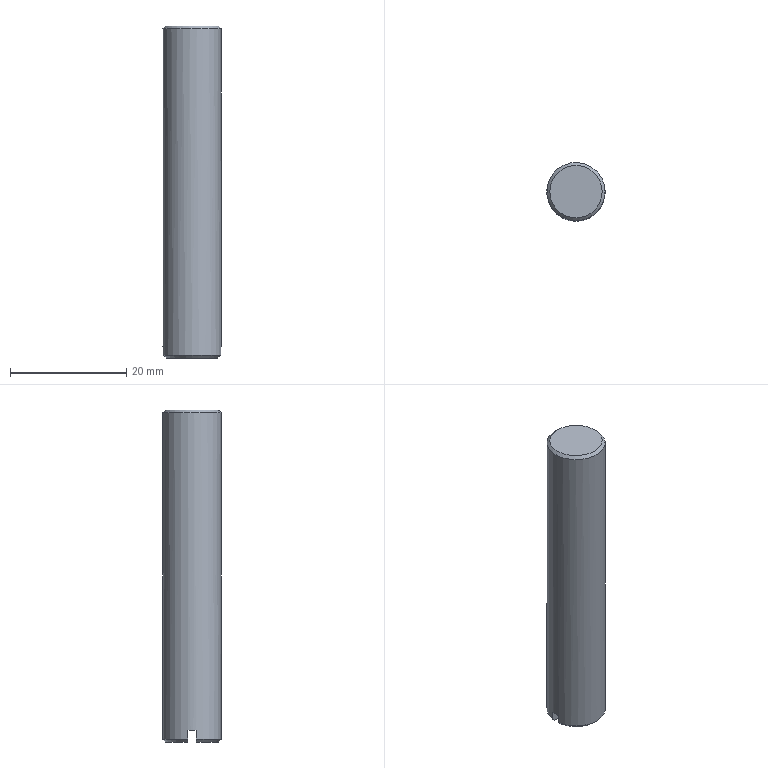Part | NX | 1 solid | 10 faces | box 10 x 10 x 57 mm | volume 4440 mm3 | plane 6 | cone 3 | cylinder 1 | commonest cylinder face diameters 10 x1
STEP:
#1=CARTESIAN_POINT('',(4.437,-0.75,-28.5));
#2=VERTEX_POINT('',#1);
#3=CARTESIAN_POINT('',(-4.437,-0.75,-28.5));
#4=VERTEX_POINT('',#3);
#5=CARTESIAN_POINT('',(0.,0.,-28.5));
#6=DIRECTION('',(0.,0.,1.));
#7=DIRECTION('',(1.,0.,0.));
#8=AXIS2_PLACEMENT_3D('',#5,#6,#7);
#9=CIRCLE('',#8,4.5);
#10=EDGE_CURVE('',#2,#4,#9,.F.);
#11=ORIENTED_EDGE('',*,*,#10,.T.);
#12=CARTESIAN_POINT('',(7.5,-0.75,-28.5));
#13=DIRECTION('',(-1.,0.,0.));
#14=VECTOR('',#13,1000.);
#15=LINE('',#12,#14);
#16=EDGE_CURVE('',#2,#4,#15,.T.);
#17=ORIENTED_EDGE('',*,*,#16,.F.);
#18=EDGE_LOOP('',(#11,#17));
#19=FACE_BOUND('',#18,.T.);
#20=CARTESIAN_POINT('',(0.,0.,-28.5));
#21=DIRECTION('',(0.,0.,1.));
#22=DIRECTION('',(1.,0.,0.));
#23=AXIS2_PLACEMENT_3D('',#20,#21,#22);
#24=PLANE('',#23);
#25=ADVANCED_FACE('',(#19),#24,.F.);
#26=CARTESIAN_POINT('',(4.943,-0.75,-28.));
#27=VERTEX_POINT('',#26);
#28=CARTESIAN_POINT('',(4.943,-0.75,-28.));
#29=CARTESIAN_POINT('',(4.775,-0.75,-28.167));
#30=CARTESIAN_POINT('',(4.606,-0.75,-28.333));
#31=CARTESIAN_POINT('',(4.437,-0.75,-28.5));
#32=B_SPLINE_CURVE_WITH_KNOTS('',3,(#28,#29,#30,#31),.UNSPECIFIED.,.F.,.F.,(4,4),(0.008518,0.00923),.UNSPECIFIED.);
#33=EDGE_CURVE('',#27,#2,#32,.T.);
#34=ORIENTED_EDGE('',*,*,#33,.F.);
#35=CARTESIAN_POINT('',(-4.943,-0.75,-28.));
#36=VERTEX_POINT('',#35);
#37=CARTESIAN_POINT('',(0.,0.,-28.));
#38=DIRECTION('',(0.,0.,1.));
#39=DIRECTION('',(1.,0.,0.));
#40=AXIS2_PLACEMENT_3D('',#37,#38,#39);
#41=CIRCLE('',#40,5.);
#42=EDGE_CURVE('',#36,#27,#41,.T.);
#43=ORIENTED_EDGE('',*,*,#42,.F.);
#44=CARTESIAN_POINT('',(-4.437,-0.75,-28.5));
#45=CARTESIAN_POINT('',(-4.606,-0.75,-28.333));
#46=CARTESIAN_POINT('',(-4.775,-0.75,-28.167));
#47=CARTESIAN_POINT('',(-4.943,-0.75,-28.));
#48=B_SPLINE_CURVE_WITH_KNOTS('',3,(#44,#45,#46,#47),.UNSPECIFIED.,.F.,.F.,(4,4),(0.02102,0.02173),.UNSPECIFIED.);
#49=EDGE_CURVE('',#4,#36,#48,.T.);
#50=ORIENTED_EDGE('',*,*,#49,.F.);
#51=ORIENTED_EDGE('',*,*,#10,.F.);
#52=EDGE_LOOP('',(#34,#43,#50,#51));
#53=FACE_BOUND('',#52,.T.);
#54=CARTESIAN_POINT('',(0.,0.,-28.));
#55=DIRECTION('',(0.,0.,1.));
#56=DIRECTION('',(1.,0.,0.));
#57=AXIS2_PLACEMENT_3D('',#54,#55,#56);
#58=CONICAL_SURFACE('',#57,5.,0.7854);
#59=ADVANCED_FACE('',(#53),#58,.T.);
#60=CARTESIAN_POINT('',(-4.943,0.75,-26.5));
#61=VERTEX_POINT('',#60);
#62=CARTESIAN_POINT('',(-4.943,-0.75,-26.5));
#63=VERTEX_POINT('',#62);
#64=CARTESIAN_POINT('',(0.,0.,-26.5));
#65=DIRECTION('',(0.,0.,1.));
#66=DIRECTION('',(1.,0.,0.));
#67=AXIS2_PLACEMENT_3D('',#64,#65,#66);
#68=CIRCLE('',#67,5.);
#69=EDGE_CURVE('',#61,#63,#68,.T.);
#70=ORIENTED_EDGE('',*,*,#69,.T.);
#71=CARTESIAN_POINT('',(-4.943,-0.75,28.5));
#72=DIRECTION('',(0.,0.,-1.));
#73=VECTOR('',#72,1000.);
#74=LINE('',#71,#73);
#75=EDGE_CURVE('',#63,#36,#74,.T.);
#76=ORIENTED_EDGE('',*,*,#75,.T.);
#77=ORIENTED_EDGE('',*,*,#42,.T.);
#78=CARTESIAN_POINT('',(4.943,-0.75,-26.5));
#79=VERTEX_POINT('',#78);
#80=CARTESIAN_POINT('',(4.943,-0.75,28.5));
#81=DIRECTION('',(0.,0.,-1.));
#82=VECTOR('',#81,1000.);
#83=LINE('',#80,#82);
#84=EDGE_CURVE('',#27,#79,#83,.F.);
#85=ORIENTED_EDGE('',*,*,#84,.T.);
#86=CARTESIAN_POINT('',(4.943,0.75,-26.5));
#87=VERTEX_POINT('',#86);
#88=CARTESIAN_POINT('',(0.,0.,-26.5));
#89=DIRECTION('',(0.,0.,1.));
#90=DIRECTION('',(1.,0.,0.));
#91=AXIS2_PLACEMENT_3D('',#88,#89,#90);
#92=CIRCLE('',#91,5.);
#93=EDGE_CURVE('',#79,#87,#92,.T.);
#94=ORIENTED_EDGE('',*,*,#93,.T.);
#95=CARTESIAN_POINT('',(4.943,0.75,-28.));
#96=VERTEX_POINT('',#95);
#97=CARTESIAN_POINT('',(4.943,0.75,28.5));
#98=DIRECTION('',(0.,0.,-1.));
#99=VECTOR('',#98,1000.);
#100=LINE('',#97,#99);
#101=EDGE_CURVE('',#87,#96,#100,.T.);
#102=ORIENTED_EDGE('',*,*,#101,.T.);
#103=CARTESIAN_POINT('',(-4.943,0.75,-28.));
#104=VERTEX_POINT('',#103);
#105=CARTESIAN_POINT('',(0.,0.,-28.));
#106=DIRECTION('',(0.,0.,1.));
#107=DIRECTION('',(1.,0.,0.));
#108=AXIS2_PLACEMENT_3D('',#105,#106,#107);
#109=CIRCLE('',#108,5.);
#110=EDGE_CURVE('',#96,#104,#109,.T.);
#111=ORIENTED_EDGE('',*,*,#110,.T.);
#112=CARTESIAN_POINT('',(-4.943,0.75,28.5));
#113=DIRECTION('',(0.,0.,-1.));
#114=VECTOR('',#113,1000.);
#115=LINE('',#112,#114);
#116=EDGE_CURVE('',#104,#61,#115,.F.);
#117=ORIENTED_EDGE('',*,*,#116,.T.);
#118=EDGE_LOOP('',(#70,#76,#77,#85,#94,#102,#111,#117));
#119=FACE_BOUND('',#118,.T.);
#120=CARTESIAN_POINT('',(5.,0.,28.));
#121=VERTEX_POINT('',#120);
#122=CARTESIAN_POINT('',(0.,0.,28.));
#123=DIRECTION('',(0.,0.,1.));
#124=DIRECTION('',(1.,0.,0.));
#125=AXIS2_PLACEMENT_3D('',#122,#123,#124);
#126=CIRCLE('',#125,5.);
#127=EDGE_CURVE('',#121,#121,#126,.F.);
#128=ORIENTED_EDGE('',*,*,#127,.T.);
#129=EDGE_LOOP('',(#128));
#130=FACE_BOUND('',#129,.T.);
#131=CARTESIAN_POINT('',(0.,0.,28.5));
#132=DIRECTION('',(0.,0.,-1.));
#133=DIRECTION('',(-1.,0.,0.));
#134=AXIS2_PLACEMENT_3D('',#131,#132,#133);
#135=CYLINDRICAL_SURFACE('',#134,5.);
#136=ADVANCED_FACE('',(#119,#130),#135,.T.);
#137=CARTESIAN_POINT('',(4.5,0.,28.5));
#138=VERTEX_POINT('',#137);
#139=CARTESIAN_POINT('',(0.,0.,28.5));
#140=DIRECTION('',(0.,0.,1.));
#141=DIRECTION('',(1.,0.,0.));
#142=AXIS2_PLACEMENT_3D('',#139,#140,#141);
#143=CIRCLE('',#142,4.5);
#144=EDGE_CURVE('',#138,#138,#143,.T.);
#145=ORIENTED_EDGE('',*,*,#144,.T.);
#146=EDGE_LOOP('',(#145));
#147=FACE_BOUND('',#146,.T.);
#148=CARTESIAN_POINT('',(0.,0.,28.5));
#149=DIRECTION('',(0.,0.,1.));
#150=DIRECTION('',(1.,0.,0.));
#151=AXIS2_PLACEMENT_3D('',#148,#149,#150);
#152=PLANE('',#151);
#153=ADVANCED_FACE('',(#147),#152,.T.);
#154=CARTESIAN_POINT('',(-4.437,0.75,-28.5));
#155=VERTEX_POINT('',#154);
#156=CARTESIAN_POINT('',(4.437,0.75,-28.5));
#157=VERTEX_POINT('',#156);
#158=CARTESIAN_POINT('',(0.,0.,-28.5));
#159=DIRECTION('',(0.,0.,1.));
#160=DIRECTION('',(1.,0.,0.));
#161=AXIS2_PLACEMENT_3D('',#158,#159,#160);
#162=CIRCLE('',#161,4.5);
#163=EDGE_CURVE('',#155,#157,#162,.F.);
#164=ORIENTED_EDGE('',*,*,#163,.T.);
#165=CARTESIAN_POINT('',(7.5,0.75,-28.5));
#166=DIRECTION('',(1.,0.,0.));
#167=VECTOR('',#166,1000.);
#168=LINE('',#165,#167);
#169=EDGE_CURVE('',#155,#157,#168,.T.);
#170=ORIENTED_EDGE('',*,*,#169,.F.);
#171=EDGE_LOOP('',(#164,#170));
#172=FACE_BOUND('',#171,.T.);
#173=CARTESIAN_POINT('',(0.,0.,-28.5));
#174=DIRECTION('',(0.,0.,1.));
#175=DIRECTION('',(1.,0.,0.));
#176=AXIS2_PLACEMENT_3D('',#173,#174,#175);
#177=PLANE('',#176);
#178=ADVANCED_FACE('',(#172),#177,.F.);
#179=CARTESIAN_POINT('',(-4.943,0.75,-28.));
#180=CARTESIAN_POINT('',(-4.775,0.75,-28.167));
#181=CARTESIAN_POINT('',(-4.606,0.75,-28.333));
#182=CARTESIAN_POINT('',(-4.437,0.75,-28.5));
#183=B_SPLINE_CURVE_WITH_KNOTS('',3,(#179,#180,#181,#182),.UNSPECIFIED.,.F.,.F.,(4,4),(0.008518,0.00923),.UNSPECIFIED.);
#184=EDGE_CURVE('',#104,#155,#183,.T.);
#185=ORIENTED_EDGE('',*,*,#184,.F.);
#186=ORIENTED_EDGE('',*,*,#110,.F.);
#187=CARTESIAN_POINT('',(4.437,0.75,-28.5));
#188=CARTESIAN_POINT('',(4.606,0.75,-28.333));
#189=CARTESIAN_POINT('',(4.775,0.75,-28.167));
#190=CARTESIAN_POINT('',(4.943,0.75,-28.));
#191=B_SPLINE_CURVE_WITH_KNOTS('',3,(#187,#188,#189,#190),.UNSPECIFIED.,.F.,.F.,(4,4),(0.02102,0.02173),.UNSPECIFIED.);
#192=EDGE_CURVE('',#157,#96,#191,.T.);
#193=ORIENTED_EDGE('',*,*,#192,.F.);
#194=ORIENTED_EDGE('',*,*,#163,.F.);
#195=EDGE_LOOP('',(#185,#186,#193,#194));
#196=FACE_BOUND('',#195,.T.);
#197=CARTESIAN_POINT('',(0.,0.,-28.));
#198=DIRECTION('',(0.,0.,1.));
#199=DIRECTION('',(1.,0.,0.));
#200=AXIS2_PLACEMENT_3D('',#197,#198,#199);
#201=CONICAL_SURFACE('',#200,5.,0.7854);
#202=ADVANCED_FACE('',(#196),#201,.T.);
#203=ORIENTED_EDGE('',*,*,#127,.F.);
#204=EDGE_LOOP('',(#203));
#205=FACE_BOUND('',#204,.T.);
#206=ORIENTED_EDGE('',*,*,#144,.F.);
#207=EDGE_LOOP('',(#206));
#208=FACE_BOUND('',#207,.T.);
#209=CARTESIAN_POINT('',(0.,0.,28.5));
#210=DIRECTION('',(0.,0.,-1.));
#211=DIRECTION('',(-1.,0.,0.));
#212=AXIS2_PLACEMENT_3D('',#209,#210,#211);
#213=CONICAL_SURFACE('',#212,4.5,0.7854);
#214=ADVANCED_FACE('',(#205,#208),#213,.T.);
#215=CARTESIAN_POINT('',(7.5,0.75,-26.5));
#216=DIRECTION('',(1.,0.,0.));
#217=VECTOR('',#216,1000.);
#218=LINE('',#215,#217);
#219=EDGE_CURVE('',#61,#87,#218,.T.);
#220=ORIENTED_EDGE('',*,*,#219,.T.);
#221=ORIENTED_EDGE('',*,*,#93,.F.);
#222=CARTESIAN_POINT('',(7.5,-0.75,-26.5));
#223=DIRECTION('',(-1.,0.,0.));
#224=VECTOR('',#223,1000.);
#225=LINE('',#222,#224);
#226=EDGE_CURVE('',#79,#63,#225,.T.);
#227=ORIENTED_EDGE('',*,*,#226,.T.);
#228=ORIENTED_EDGE('',*,*,#69,.F.);
#229=EDGE_LOOP('',(#220,#221,#227,#228));
#230=FACE_BOUND('',#229,.T.);
#231=CARTESIAN_POINT('',(0.,0.,-26.5));
#232=DIRECTION('',(0.,0.,1.));
#233=DIRECTION('',(1.,0.,0.));
#234=AXIS2_PLACEMENT_3D('',#231,#232,#233);
#235=PLANE('',#234);
#236=ADVANCED_FACE('',(#230),#235,.F.);
#237=ORIENTED_EDGE('',*,*,#33,.T.);
#238=ORIENTED_EDGE('',*,*,#16,.T.);
#239=ORIENTED_EDGE('',*,*,#49,.T.);
#240=ORIENTED_EDGE('',*,*,#75,.F.);
#241=ORIENTED_EDGE('',*,*,#226,.F.);
#242=ORIENTED_EDGE('',*,*,#84,.F.);
#243=EDGE_LOOP('',(#237,#238,#239,#240,#241,#242));
#244=FACE_BOUND('',#243,.T.);
#245=CARTESIAN_POINT('',(7.5,-0.75,-26.5));
#246=DIRECTION('',(0.,-1.,0.));
#247=DIRECTION('',(0.,0.,-1.));
#248=AXIS2_PLACEMENT_3D('',#245,#246,#247);
#249=PLANE('',#248);
#250=ADVANCED_FACE('',(#244),#249,.F.);
#251=ORIENTED_EDGE('',*,*,#184,.T.);
#252=ORIENTED_EDGE('',*,*,#169,.T.);
#253=ORIENTED_EDGE('',*,*,#192,.T.);
#254=ORIENTED_EDGE('',*,*,#101,.F.);
#255=ORIENTED_EDGE('',*,*,#219,.F.);
#256=ORIENTED_EDGE('',*,*,#116,.F.);
#257=EDGE_LOOP('',(#251,#252,#253,#254,#255,#256));
#258=FACE_BOUND('',#257,.T.);
#259=CARTESIAN_POINT('',(7.5,0.75,-26.5));
#260=DIRECTION('',(0.,1.,0.));
#261=DIRECTION('',(0.,0.,1.));
#262=AXIS2_PLACEMENT_3D('',#259,#260,#261);
#263=PLANE('',#262);
#264=ADVANCED_FACE('',(#258),#263,.F.);
#265=CLOSED_SHELL('',(#25,#59,#136,#153,#178,#202,#214,#236,#250,#264));
#266=MANIFOLD_SOLID_BREP('',#265);
#267=(LENGTH_UNIT()NAMED_UNIT(*)SI_UNIT(.MILLI.,.METRE.));
#268=UNCERTAINTY_MEASURE_WITH_UNIT(LENGTH_MEASURE(0.0508),#267,'','');
#269=(NAMED_UNIT(*)PLANE_ANGLE_UNIT()SI_UNIT($,.RADIAN.));
#270=(NAMED_UNIT(*)SI_UNIT($,.STERADIAN.)SOLID_ANGLE_UNIT());
#271=(GEOMETRIC_REPRESENTATION_CONTEXT(3)GLOBAL_UNCERTAINTY_ASSIGNED_CONTEXT((#268))GLOBAL_UNIT_ASSIGNED_CONTEXT((#267,#269,#270))REPRESENTATION_CONTEXT('',''));
#272=ADVANCED_BREP_SHAPE_REPRESENTATION('',(#266),#271);